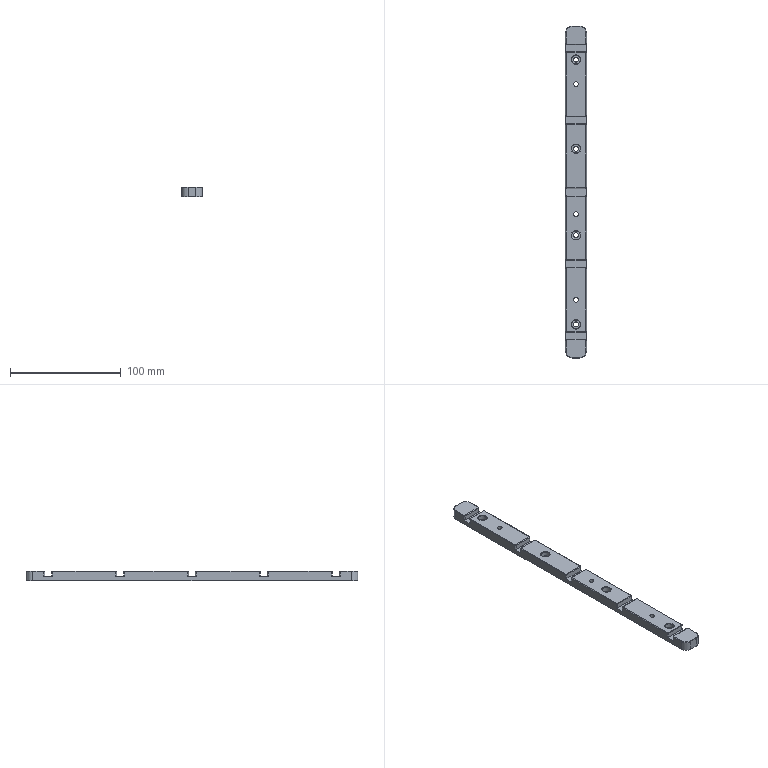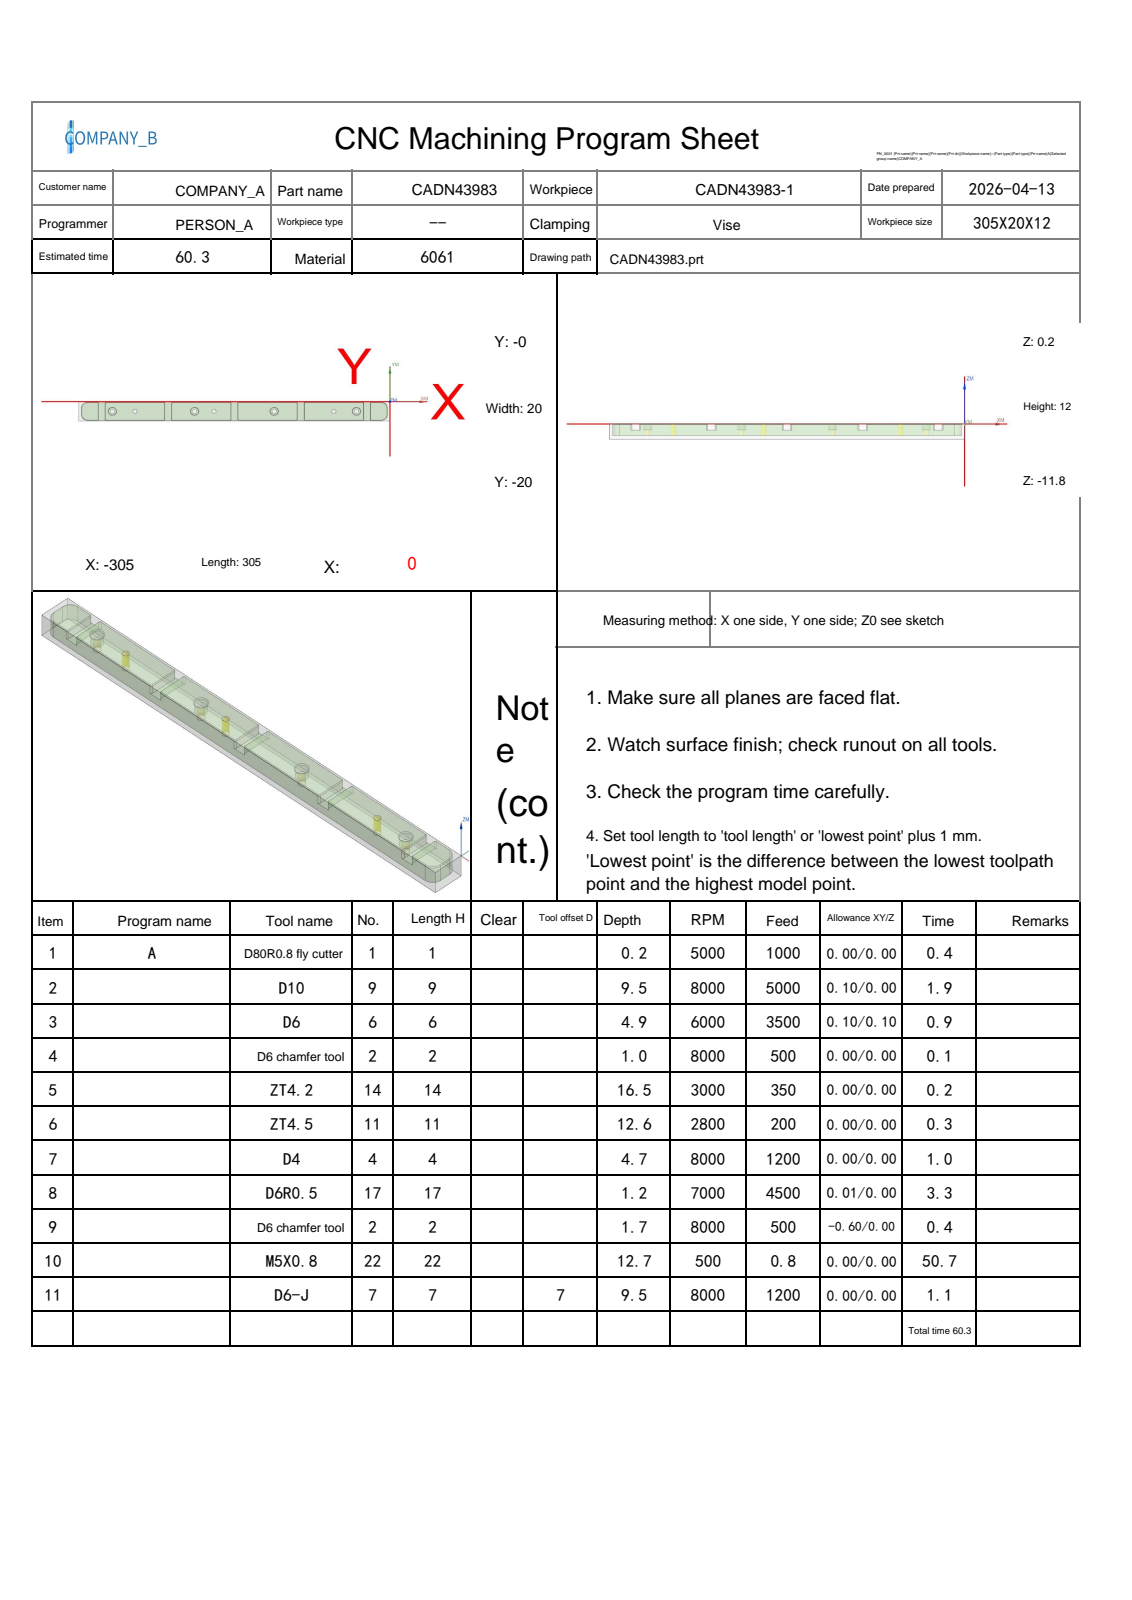NC program | NX | posted by the shop | part box 19 x 300 x 9 mm
Lines 1 to 1453 of 20188:
%
O0001
(Machine time: 109.25 MIN)
(===Total Tool:10===)
(T1=D80R0.8 fly cutter D=80.  R=0.8  D-  H01 Z=-0.   )
(T9=D10     D=10.  R=0.   D-  H09 Z=-9.3  )
(T6=D6      D=6.   R=0.   D-  H06 Z=-4.7  )
(T2=D6 chamfer tool   D=6.   R=0.   D-  H02 Z=-1.5  )
(T14=ZT4.2  D=4.2  DR_a=118 D-  H14 Z=-16.26)
(T11=ZT4.5  D=4.5  DR_a=118 D-  H11 Z=-12.35)
(T4=D4      D=4.   R=0.   D4  H04 Z=-4.5  )
(T17=D6R0.5 D=6.   R=0.5  D-  H17 Z=-1.   )
(T22=M5X0.8 D=4.2  DR_a=180 D-  H22 Z=-12.5 )
(T7=D6-J    D=6.   R=0.   D7  H07 Z=-9.3  )
G80 G90 G17 G49 G40
G91 G28 Z0
M01
N1 T01 M06
(D80R0.8 fly cutter  D=80. R=0.8 H=01 ce=0.00 di=0.00)
G00 G90 G54 X-347.5 Y-10. M03 S5000
G43 H01 Z20.
M08
Z2.
G01 Z0.0 F1000.
X-342.5
X37.5
X42.5
Z2.
G00 Z20.
G91 G28 Z0.0
M05
M09
G91 G28 Z0.0
M01
N2 T09 M06
(D10  D=10. R=0. H=09 ce=0.10 di=0.00)
G00 G90 G54 X-152.5 Y-24.6 M03 S8000
G43 H09 Z20.
M08
Z.5
G01 X-296.5 Z.335 F5000.
G02 X-307.6 Y-13.5 Z.316 I0.0 J11.1
G01 Y-6.5 Z.308
G02 X-296.5 Y4.6 Z.288 I11.1 J0.0
G01 X-8.5 Z-.041
G02 X2.6 Y-6.5 Z-.061 I0.0 J-11.1
G01 Y-13.5 Z-.069
G02 X-8.5 Y-24.6 Z-.089 I-11.1 J0.0
G01 X-296.5 Z-.418
G02 X-307.6 Y-13.5 Z-.438 I0.0 J11.1
G01 Y-6.5 Z-.446
G02 X-296.5 Y4.6 Z-.466 I11.1 J0.0
G01 X-8.5 Z-.795
G02 X2.6 Y-6.5 Z-.815 I0.0 J-11.1
G01 Y-13.5 Z-.823
G02 X-8.5 Y-24.6 Z-.843 I-11.1 J0.0
G01 X-296.5 Z-1.172
G02 X-307.6 Y-13.5 Z-1.192 I0.0 J11.1
G01 Y-6.5 Z-1.2
G02 X-296.5 Y4.6 Z-1.22 I11.1 J0.0
G01 X-8.5 Z-1.549
G02 X2.6 Y-6.5 Z-1.569 I0.0 J-11.1
G01 Y-13.5 Z-1.577
G02 X-8.5 Y-24.6 Z-1.597 I-11.1 J0.0
G01 X-296.5 Z-1.926
G02 X-307.6 Y-13.5 Z-1.946 I0.0 J11.1
G01 Y-6.5 Z-1.954
G02 X-296.5 Y4.6 Z-1.974 I11.1 J0.0
G01 X-8.5 Z-2.303
G02 X2.6 Y-6.5 Z-2.323 I0.0 J-11.1
G01 Y-13.5 Z-2.331
G02 X-8.5 Y-24.6 Z-2.351 I-11.1 J0.0
G01 X-296.5 Z-2.68
G02 X-307.6 Y-13.5 Z-2.7 I0.0 J11.1
G01 Y-6.5 Z-2.708
G02 X-296.5 Y4.6 Z-2.728 I11.1 J0.0
G01 X-8.5 Z-3.057
G02 X2.6 Y-6.5 Z-3.077 I0.0 J-11.1
G01 Y-13.5 Z-3.085
G02 X-8.5 Y-24.6 Z-3.105 I-11.1 J0.0
G01 X-296.5 Z-3.434
G02 X-307.6 Y-13.5 Z-3.454 I0.0 J11.1
G01 Y-6.5 Z-3.462
G02 X-296.5 Y4.6 Z-3.482 I11.1 J0.0
G01 X-8.5 Z-3.811
G02 X2.6 Y-6.5 Z-3.831 I0.0 J-11.1
G01 Y-13.5 Z-3.839
G02 X-8.5 Y-24.6 Z-3.859 I-11.1 J0.0
G01 X-296.5 Z-4.188
G02 X-307.6 Y-13.5 Z-4.208 I0.0 J11.1
G01 Y-6.5 Z-4.216
G02 X-296.5 Y4.6 Z-4.235 I11.1 J0.0
G01 X-8.5 Z-4.565
G02 X2.6 Y-6.5 Z-4.584 I0.0 J-11.1
G01 Y-13.5 Z-4.592
G02 X-8.5 Y-24.6 Z-4.612 I-11.1 J0.0
G01 X-296.5 Z-4.941
G02 X-307.6 Y-13.5 Z-4.961 I0.0 J11.1
G01 Y-6.5 Z-4.969
G02 X-296.5 Y4.6 Z-4.989 I11.1 J0.0
G01 X-8.5 Z-5.318
G02 X2.6 Y-6.5 Z-5.338 I0.0 J-11.1
G01 Y-13.5 Z-5.346
G02 X-8.5 Y-24.6 Z-5.366 I-11.1 J0.0
G01 X-296.5 Z-5.695
G02 X-307.6 Y-13.5 Z-5.715 I0.0 J11.1
G01 Y-6.5 Z-5.723
G02 X-296.5 Y4.6 Z-5.743 I11.1 J0.0
G01 X-8.5 Z-6.072
G02 X2.6 Y-6.5 Z-6.092 I0.0 J-11.1
G01 Y-13.5 Z-6.1
G02 X-8.5 Y-24.6 Z-6.12 I-11.1 J0.0
G01 X-296.5 Z-6.449
G02 X-307.6 Y-13.5 Z-6.469 I0.0 J11.1
G01 Y-6.5 Z-6.477
G02 X-296.5 Y4.6 Z-6.497 I11.1 J0.0
G01 X-8.5 Z-6.826
G02 X2.6 Y-6.5 Z-6.846 I0.0 J-11.1
G01 Y-13.5 Z-6.854
G02 X-8.5 Y-24.6 Z-6.874 I-11.1 J0.0
G01 X-296.5 Z-7.203
G02 X-307.6 Y-13.5 Z-7.223 I0.0 J11.1
G01 Y-6.5 Z-7.231
G02 X-296.5 Y4.6 Z-7.251 I11.1 J0.0
G01 X-8.5 Z-7.58
G02 X2.6 Y-6.5 Z-7.6 I0.0 J-11.1
G01 Y-13.5 Z-7.608
G02 X-8.5 Y-24.6 Z-7.628 I-11.1 J0.0
G01 X-296.5 Z-7.957
G02 X-307.6 Y-13.5 Z-7.977 I0.0 J11.1
G01 Y-6.5 Z-7.985
G02 X-296.5 Y4.6 Z-8.005 I11.1 J0.0
G01 X-8.5 Z-8.334
G02 X2.6 Y-6.5 Z-8.354 I0.0 J-11.1
G01 Y-13.5 Z-8.362
G02 X-8.5 Y-24.6 Z-8.382 I-11.1 J0.0
G01 X-296.5 Z-8.711
G02 X-307.6 Y-13.5 Z-8.731 I0.0 J11.1
G01 Y-6.5 Z-8.739
G02 X-296.5 Y4.6 Z-8.759 I11.1 J0.0
G01 X-8.5 Z-9.088
G02 X2.6 Y-6.5 Z-9.108 I0.0 J-11.1
G01 Y-13.5 Z-9.116
G02 X-8.5 Y-24.6 Z-9.135 I-11.1 J0.0
G01 X-152.5 Z-9.3
X-296.5
G02 X-307.6 Y-13.5 I0.0 J11.1
G01 Y-6.5
G02 X-296.5 Y4.6 I11.1 J0.0
G01 X-8.5
G02 X2.6 Y-6.5 I0.0 J-11.1
G01 Y-13.5
G02 X-8.5 Y-24.6 I-11.1 J0.0
G01 X-152.5
X-153.
Z-8.3
G00 Z20.
G91 G28 Z0.0
M05
M09
G91 G28 Z0.0
M01
N3 T06 M06
(D6  D=6. R=0. H=06 ce=0.10 di=0.10)
G00 G90 G54 X-22.5 Y5.5 M03 S6000
G43 H06 Z20.
M08
Z.108
G01 Z-.392 F3500.
Y.1
X-22.875
G02 X-22.55 Y-1.5 I-3.775 J-1.6
G01 Y-18.5
G02 X-22.875 Y-20.1 I-4.1 J0.0
G01 X-22.125
G02 X-22.45 Y-18.5 I3.775 J1.6
G01 Y-1.5
G02 X-22.125 Y.1 I4.1 J0.0
G01 X-22.5
X-22.875
X-22.828 Y-.016
Z.108
G00 Z.5
X-22.5 Y5.5
Z-.283
G01 Z-.783
Y.1
X-22.875
G02 X-22.55 Y-1.5 I-3.775 J-1.6
G01 Y-18.5
G02 X-22.875 Y-20.1 I-4.1 J0.0
G01 X-22.125
G02 X-22.45 Y-18.5 I3.775 J1.6
G01 Y-1.5
G02 X-22.125 Y.1 I4.1 J0.0
G01 X-22.5
X-22.875
X-22.828 Y-.016
Z-.283
G00 Z.108
X-22.5 Y5.5
Z-.675
G01 Z-1.175
Y.1
X-22.875
G02 X-22.55 Y-1.5 I-3.775 J-1.6
G01 Y-18.5
G02 X-22.875 Y-20.1 I-4.1 J0.0
G01 X-22.125
G02 X-22.45 Y-18.5 I3.775 J1.6
G01 Y-1.5
G02 X-22.125 Y.1 I4.1 J0.0
G01 X-22.5
X-22.875
X-22.828 Y-.016
Z-.675
G00 Z-.283
X-22.5 Y5.5
Z-1.067
G01 Z-1.567
Y.1
X-22.875
G02 X-22.55 Y-1.5 I-3.775 J-1.6
G01 Y-18.5
G02 X-22.875 Y-20.1 I-4.1 J0.0
G01 X-22.125
G02 X-22.45 Y-18.5 I3.775 J1.6
G01 Y-1.5
G02 X-22.125 Y.1 I4.1 J0.0
G01 X-22.5
X-22.875
X-22.828 Y-.016
Z-1.067
G00 Z-.675
X-22.5 Y5.5
Z-1.458
G01 Z-1.958
Y.1
X-22.875
G02 X-22.55 Y-1.5 I-3.775 J-1.6
G01 Y-18.5
G02 X-22.875 Y-20.1 I-4.1 J0.0
G01 X-22.125
G02 X-22.45 Y-18.5 I3.775 J1.6
G01 Y-1.5
G02 X-22.125 Y.1 I4.1 J0.0
G01 X-22.5
X-22.875
X-22.828 Y-.016
Z-1.458
G00 Z-1.067
X-22.5 Y5.5
Z-1.85
G01 Z-2.35
Y.1
X-22.875
G02 X-22.55 Y-1.5 I-3.775 J-1.6
G01 Y-18.5
G02 X-22.875 Y-20.1 I-4.1 J0.0
G01 X-22.125
G02 X-22.45 Y-18.5 I3.775 J1.6
G01 Y-1.5
G02 X-22.125 Y.1 I4.1 J0.0
G01 X-22.5
X-22.875
X-22.828 Y-.016
Z-1.85
G00 Z-1.458
X-22.5 Y5.5
Z-2.242
G01 Z-2.742
Y.1
X-22.875
G02 X-22.55 Y-1.5 I-3.775 J-1.6
G01 Y-18.5
G02 X-22.875 Y-20.1 I-4.1 J0.0
G01 X-22.125
G02 X-22.45 Y-18.5 I3.775 J1.6
G01 Y-1.5
G02 X-22.125 Y.1 I4.1 J0.0
G01 X-22.5
X-22.875
X-22.828 Y-.016
Z-2.242
G00 Z-1.85
X-22.5 Y5.5
Z-2.633
G01 Z-3.133
Y.1
X-22.875
G02 X-22.55 Y-1.5 I-3.775 J-1.6
G01 Y-18.5
G02 X-22.875 Y-20.1 I-4.1 J0.0
G01 X-22.125
G02 X-22.45 Y-18.5 I3.775 J1.6
G01 Y-1.5
G02 X-22.125 Y.1 I4.1 J0.0
G01 X-22.5
X-22.875
X-22.828 Y-.016
Z-2.633
G00 Z-2.242
X-22.5 Y5.5
Z-3.025
G01 Z-3.525
Y.1
X-22.875
G02 X-22.55 Y-1.5 I-3.775 J-1.6
G01 Y-18.5
G02 X-22.875 Y-20.1 I-4.1 J0.0
G01 X-22.125
G02 X-22.45 Y-18.5 I3.775 J1.6
G01 Y-1.5
G02 X-22.125 Y.1 I4.1 J0.0
G01 X-22.5
X-22.875
X-22.828 Y-.016
Z-3.025
G00 Z-2.633
X-22.5 Y5.5
Z-3.417
G01 Z-3.917
Y.1
X-22.875
G02 X-22.55 Y-1.5 I-3.775 J-1.6
G01 Y-18.5
G02 X-22.875 Y-20.1 I-4.1 J0.0
G01 X-22.125
G02 X-22.45 Y-18.5 I3.775 J1.6
G01 Y-1.5
G02 X-22.125 Y.1 I4.1 J0.0
G01 X-22.5
X-22.875
X-22.828 Y-.016
Z-3.417
G00 Z-3.025
X-22.5 Y5.5
Z-3.808
G01 Z-4.308
Y.1
X-22.875
G02 X-22.55 Y-1.5 I-3.775 J-1.6
G01 Y-18.5
G02 X-22.875 Y-20.1 I-4.1 J0.0
G01 X-22.125
G02 X-22.45 Y-18.5 I3.775 J1.6
G01 Y-1.5
G02 X-22.125 Y.1 I4.1 J0.0
G01 X-22.5
X-22.875
X-22.828 Y-.016
Z-3.808
G00 Z-3.417
X-22.5 Y5.5
Z-4.2
G01 Z-4.7
Y.1
X-22.875
G02 X-22.55 Y-1.5 I-3.775 J-1.6
G01 Y-18.5
G02 X-22.875 Y-20.1 I-4.1 J0.0
G01 X-22.125
G02 X-22.45 Y-18.5 I3.775 J1.6
G01 Y-1.5
G02 X-22.125 Y.1 I4.1 J0.0
G01 X-22.5
X-22.875
X-22.828 Y-.016
Z-4.2
G00 Z20.
X-87.5 Y5.5
Z.108
G01 Z-.392
Y.1
X-87.875
G02 X-87.55 Y-1.5 I-3.775 J-1.6
G01 Y-18.5
G02 X-87.875 Y-20.1 I-4.1 J0.0
G01 X-87.125
G02 X-87.45 Y-18.5 I3.775 J1.6
G01 Y-1.5
G02 X-87.125 Y.1 I4.1 J0.0
G01 X-87.5
X-87.875
X-87.828 Y-.016
Z.108
G00 Z.5
X-87.5 Y5.5
Z-.283
G01 Z-.783
Y.1
X-87.875
G02 X-87.55 Y-1.5 I-3.775 J-1.6
G01 Y-18.5
G02 X-87.875 Y-20.1 I-4.1 J0.0
G01 X-87.125
G02 X-87.45 Y-18.5 I3.775 J1.6
G01 Y-1.5
G02 X-87.125 Y.1 I4.1 J0.0
G01 X-87.5
X-87.875
X-87.828 Y-.016
Z-.283
G00 Z.108
X-87.5 Y5.5
Z-.675
G01 Z-1.175
Y.1
X-87.875
G02 X-87.55 Y-1.5 I-3.775 J-1.6
G01 Y-18.5
G02 X-87.875 Y-20.1 I-4.1 J0.0
G01 X-87.125
G02 X-87.45 Y-18.5 I3.775 J1.6
G01 Y-1.5
G02 X-87.125 Y.1 I4.1 J0.0
G01 X-87.5
X-87.875
X-87.828 Y-.016
Z-.675
G00 Z-.283
X-87.5 Y5.5
Z-1.067
G01 Z-1.567
Y.1
X-87.875
G02 X-87.55 Y-1.5 I-3.775 J-1.6
G01 Y-18.5
G02 X-87.875 Y-20.1 I-4.1 J0.0
G01 X-87.125
G02 X-87.45 Y-18.5 I3.775 J1.6
G01 Y-1.5
G02 X-87.125 Y.1 I4.1 J0.0
G01 X-87.5
X-87.875
X-87.828 Y-.016
Z-1.067
G00 Z-.675
X-87.5 Y5.5
Z-1.458
G01 Z-1.958
Y.1
X-87.875
G02 X-87.55 Y-1.5 I-3.775 J-1.6
G01 Y-18.5
G02 X-87.875 Y-20.1 I-4.1 J0.0
G01 X-87.125
G02 X-87.45 Y-18.5 I3.775 J1.6
G01 Y-1.5
G02 X-87.125 Y.1 I4.1 J0.0
G01 X-87.5
X-87.875
X-87.828 Y-.016
Z-1.458
G00 Z-1.067
X-87.5 Y5.5
Z-1.85
G01 Z-2.35
Y.1
X-87.875
G02 X-87.55 Y-1.5 I-3.775 J-1.6
G01 Y-18.5
G02 X-87.875 Y-20.1 I-4.1 J0.0
G01 X-87.125
G02 X-87.45 Y-18.5 I3.775 J1.6
G01 Y-1.5
G02 X-87.125 Y.1 I4.1 J0.0
G01 X-87.5
X-87.875
X-87.828 Y-.016
Z-1.85
G00 Z-1.458
X-87.5 Y5.5
Z-2.242
G01 Z-2.742
Y.1
X-87.875
G02 X-87.55 Y-1.5 I-3.775 J-1.6
G01 Y-18.5
G02 X-87.875 Y-20.1 I-4.1 J0.0
G01 X-87.125
G02 X-87.45 Y-18.5 I3.775 J1.6
G01 Y-1.5
G02 X-87.125 Y.1 I4.1 J0.0
G01 X-87.5
X-87.875
X-87.828 Y-.016
Z-2.242
G00 Z-1.85
X-87.5 Y5.5
Z-2.633
G01 Z-3.133
Y.1
X-87.875
G02 X-87.55 Y-1.5 I-3.775 J-1.6
G01 Y-18.5
G02 X-87.875 Y-20.1 I-4.1 J0.0
G01 X-87.125
G02 X-87.45 Y-18.5 I3.775 J1.6
G01 Y-1.5
G02 X-87.125 Y.1 I4.1 J0.0
G01 X-87.5
X-87.875
X-87.828 Y-.016
Z-2.633
G00 Z-2.242
X-87.5 Y5.5
Z-3.025
G01 Z-3.525
Y.1
X-87.875
G02 X-87.55 Y-1.5 I-3.775 J-1.6
G01 Y-18.5
G02 X-87.875 Y-20.1 I-4.1 J0.0
G01 X-87.125
G02 X-87.45 Y-18.5 I3.775 J1.6
G01 Y-1.5
G02 X-87.125 Y.1 I4.1 J0.0
G01 X-87.5
X-87.875
X-87.828 Y-.016
Z-3.025
G00 Z-2.633
X-87.5 Y5.5
Z-3.417
G01 Z-3.917
Y.1
X-87.875
G02 X-87.55 Y-1.5 I-3.775 J-1.6
G01 Y-18.5
G02 X-87.875 Y-20.1 I-4.1 J0.0
G01 X-87.125
G02 X-87.45 Y-18.5 I3.775 J1.6
G01 Y-1.5
G02 X-87.125 Y.1 I4.1 J0.0
G01 X-87.5
X-87.875
X-87.828 Y-.016
Z-3.417
G00 Z-3.025
X-87.5 Y5.5
Z-3.808
G01 Z-4.308
Y.1
X-87.875
G02 X-87.55 Y-1.5 I-3.775 J-1.6
G01 Y-18.5
G02 X-87.875 Y-20.1 I-4.1 J0.0
G01 X-87.125
G02 X-87.45 Y-18.5 I3.775 J1.6
G01 Y-1.5
G02 X-87.125 Y.1 I4.1 J0.0
G01 X-87.5
X-87.875
X-87.828 Y-.016
Z-3.808
G00 Z-3.417
X-87.5 Y5.5
Z-4.2
G01 Z-4.7
Y.1
X-87.875
G02 X-87.55 Y-1.5 I-3.775 J-1.6
G01 Y-18.5
G02 X-87.875 Y-20.1 I-4.1 J0.0
G01 X-87.125
G02 X-87.45 Y-18.5 I3.775 J1.6
G01 Y-1.5
G02 X-87.125 Y.1 I4.1 J0.0
G01 X-87.5
X-87.875
X-87.828 Y-.016
Z-4.2
G00 Z20.
X-152.5 Y5.5
Z.108
G01 Z-.392
Y.1
X-152.875
G02 X-152.55 Y-1.5 I-3.775 J-1.6
G01 Y-18.5
G02 X-152.875 Y-20.1 I-4.1 J0.0
G01 X-152.125
G02 X-152.45 Y-18.5 I3.775 J1.6
G01 Y-1.5
G02 X-152.125 Y.1 I4.1 J0.0
G01 X-152.5
X-152.875
X-152.828 Y-.016
Z.108
G00 Z.5
X-152.5 Y5.5
Z-.283
G01 Z-.783
Y.1
X-152.875
G02 X-152.55 Y-1.5 I-3.775 J-1.6
G01 Y-18.5
G02 X-152.875 Y-20.1 I-4.1 J0.0
G01 X-152.125
G02 X-152.45 Y-18.5 I3.775 J1.6
G01 Y-1.5
G02 X-152.125 Y.1 I4.1 J0.0
G01 X-152.5
X-152.875
X-152.828 Y-.016
Z-.283
G00 Z.108
X-152.5 Y5.5
Z-.675
G01 Z-1.175
Y.1
X-152.875
G02 X-152.55 Y-1.5 I-3.775 J-1.6
G01 Y-18.5
G02 X-152.875 Y-20.1 I-4.1 J0.0
G01 X-152.125
G02 X-152.45 Y-18.5 I3.775 J1.6
G01 Y-1.5
G02 X-152.125 Y.1 I4.1 J0.0
G01 X-152.5
X-152.875
X-152.828 Y-.016
Z-.675
G00 Z-.283
X-152.5 Y5.5
Z-1.067
G01 Z-1.567
Y.1
X-152.875
G02 X-152.55 Y-1.5 I-3.775 J-1.6
G01 Y-18.5
G02 X-152.875 Y-20.1 I-4.1 J0.0
G01 X-152.125
G02 X-152.45 Y-18.5 I3.775 J1.6
G01 Y-1.5
G02 X-152.125 Y.1 I4.1 J0.0
G01 X-152.5
X-152.875
X-152.828 Y-.016
Z-1.067
G00 Z-.675
X-152.5 Y5.5
Z-1.458
G01 Z-1.958
Y.1
X-152.875
G02 X-152.55 Y-1.5 I-3.775 J-1.6
G01 Y-18.5
G02 X-152.875 Y-20.1 I-4.1 J0.0
G01 X-152.125
G02 X-152.45 Y-18.5 I3.775 J1.6
G01 Y-1.5
G02 X-152.125 Y.1 I4.1 J0.0
G01 X-152.5
X-152.875
X-152.828 Y-.016
Z-1.458
G00 Z-1.067
X-152.5 Y5.5
Z-1.85
G01 Z-2.35
Y.1
X-152.875
G02 X-152.55 Y-1.5 I-3.775 J-1.6
G01 Y-18.5
G02 X-152.875 Y-20.1 I-4.1 J0.0
G01 X-152.125
G02 X-152.45 Y-18.5 I3.775 J1.6
G01 Y-1.5
G02 X-152.125 Y.1 I4.1 J0.0
G01 X-152.5
X-152.875
X-152.828 Y-.016
Z-1.85
G00 Z-1.458
X-152.5 Y5.5
Z-2.242
G01 Z-2.742
Y.1
X-152.875
G02 X-152.55 Y-1.5 I-3.775 J-1.6
G01 Y-18.5
G02 X-152.875 Y-20.1 I-4.1 J0.0
G01 X-152.125
G02 X-152.45 Y-18.5 I3.775 J1.6
G01 Y-1.5
G02 X-152.125 Y.1 I4.1 J0.0
G01 X-152.5
X-152.875
X-152.828 Y-.016
Z-2.242
G00 Z-1.85
X-152.5 Y5.5
Z-2.633
G01 Z-3.133
Y.1
X-152.875
G02 X-152.55 Y-1.5 I-3.775 J-1.6
G01 Y-18.5
G02 X-152.875 Y-20.1 I-4.1 J0.0
G01 X-152.125
G02 X-152.45 Y-18.5 I3.775 J1.6
G01 Y-1.5
G02 X-152.125 Y.1 I4.1 J0.0
G01 X-152.5
X-152.875
X-152.828 Y-.016
Z-2.633
G00 Z-2.242
X-152.5 Y5.5
Z-3.025
G01 Z-3.525
Y.1
X-152.875
G02 X-152.55 Y-1.5 I-3.775 J-1.6
G01 Y-18.5
G02 X-152.875 Y-20.1 I-4.1 J0.0
G01 X-152.125
G02 X-152.45 Y-18.5 I3.775 J1.6
G01 Y-1.5
G02 X-152.125 Y.1 I4.1 J0.0
G01 X-152.5
X-152.875
X-152.828 Y-.016
Z-3.025
G00 Z-2.633
X-152.5 Y5.5
Z-3.417
G01 Z-3.917
Y.1
X-152.875
G02 X-152.55 Y-1.5 I-3.775 J-1.6
G01 Y-18.5
G02 X-152.875 Y-20.1 I-4.1 J0.0
G01 X-152.125
G02 X-152.45 Y-18.5 I3.775 J1.6
G01 Y-1.5
G02 X-152.125 Y.1 I4.1 J0.0
G01 X-152.5
X-152.875
X-152.828 Y-.016
Z-3.417
G00 Z-3.025
X-152.5 Y5.5
Z-3.808
G01 Z-4.308
Y.1
X-152.875
G02 X-152.55 Y-1.5 I-3.775 J-1.6
G01 Y-18.5
G02 X-152.875 Y-20.1 I-4.1 J0.0
G01 X-152.125
G02 X-152.45 Y-18.5 I3.775 J1.6
G01 Y-1.5
G02 X-152.125 Y.1 I4.1 J0.0
G01 X-152.5
X-152.875
X-152.828 Y-.016
Z-3.808
G00 Z-3.417
X-152.5 Y5.5
Z-4.2
G01 Z-4.7
Y.1
X-152.875
G02 X-152.55 Y-1.5 I-3.775 J-1.6
G01 Y-18.5
G02 X-152.875 Y-20.1 I-4.1 J0.0
G01 X-152.125
G02 X-152.45 Y-18.5 I3.775 J1.6
G01 Y-1.5
G02 X-152.125 Y.1 I4.1 J0.0
G01 X-152.5
X-152.875
X-152.828 Y-.016
Z-4.2
G00 Z20.
X-217.5 Y5.5
Z.108
G01 Z-.392
Y.1
X-217.875
G02 X-217.55 Y-1.5 I-3.775 J-1.6
G01 Y-18.5
G02 X-217.875 Y-20.1 I-4.1 J0.0
G01 X-217.125
G02 X-217.45 Y-18.5 I3.775 J1.6
G01 Y-1.5
G02 X-217.125 Y.1 I4.1 J0.0
G01 X-217.5
X-217.875
X-217.828 Y-.016
Z.108
G00 Z.5
X-217.5 Y5.5
Z-.283
G01 Z-.783
Y.1
X-217.875
G02 X-217.55 Y-1.5 I-3.775 J-1.6
G01 Y-18.5
G02 X-217.875 Y-20.1 I-4.1 J0.0
G01 X-217.125
G02 X-217.45 Y-18.5 I3.775 J1.6
G01 Y-1.5
G02 X-217.125 Y.1 I4.1 J0.0
G01 X-217.5
X-217.875
X-217.828 Y-.016
Z-.283
G00 Z.108
X-217.5 Y5.5
Z-.675
G01 Z-1.175
Y.1
X-217.875
G02 X-217.55 Y-1.5 I-3.775 J-1.6
G01 Y-18.5
G02 X-217.875 Y-20.1 I-4.1 J0.0
G01 X-217.125
G02 X-217.45 Y-18.5 I3.775 J1.6
G01 Y-1.5
G02 X-217.125 Y.1 I4.1 J0.0
G01 X-217.5
X-217.875
X-217.828 Y-.016
Z-.675
G00 Z-.283
X-217.5 Y5.5
Z-1.067
G01 Z-1.567
Y.1
X-217.875
G02 X-217.55 Y-1.5 I-3.775 J-1.6
G01 Y-18.5
G02 X-217.875 Y-20.1 I-4.1 J0.0
G01 X-217.125
G02 X-217.45 Y-18.5 I3.775 J1.6
G01 Y-1.5
G02 X-217.125 Y.1 I4.1 J0.0
G01 X-217.5
X-217.875
X-217.828 Y-.016
Z-1.067
G00 Z-.675
X-217.5 Y5.5
Z-1.458
G01 Z-1.958
Y.1
X-217.875
G02 X-217.55 Y-1.5 I-3.775 J-1.6
G01 Y-18.5
G02 X-217.875 Y-20.1 I-4.1 J0.0
G01 X-217.125
G02 X-217.45 Y-18.5 I3.775 J1.6
G01 Y-1.5
G02 X-217.125 Y.1 I4.1 J0.0
G01 X-217.5
X-217.875
X-217.828 Y-.016
Z-1.458
G00 Z-1.067
X-217.5 Y5.5
Z-1.85
G01 Z-2.35
Y.1
X-217.875
G02 X-217.55 Y-1.5 I-3.775 J-1.6
G01 Y-18.5
G02 X-217.875 Y-20.1 I-4.1 J0.0
G01 X-217.125
G02 X-217.45 Y-18.5 I3.775 J1.6
G01 Y-1.5
G02 X-217.125 Y.1 I4.1 J0.0
G01 X-217.5
X-217.875
X-217.828 Y-.016
Z-1.85
G00 Z-1.458
X-217.5 Y5.5
Z-2.242
G01 Z-2.742
Y.1
X-217.875
G02 X-217.55 Y-1.5 I-3.775 J-1.6
G01 Y-18.5
G02 X-217.875 Y-20.1 I-4.1 J0.0
G01 X-217.125
G02 X-217.45 Y-18.5 I3.775 J1.6
G01 Y-1.5
G02 X-217.125 Y.1 I4.1 J0.0
G01 X-217.5
X-217.875
X-217.828 Y-.016
Z-2.242
G00 Z-1.85
X-217.5 Y5.5
Z-2.633
G01 Z-3.133
Y.1
X-217.875
G02 X-217.55 Y-1.5 I-3.775 J-1.6
G01 Y-18.5
G02 X-217.875 Y-20.1 I-4.1 J0.0
G01 X-217.125
G02 X-217.45 Y-18.5 I3.775 J1.6
G01 Y-1.5
G02 X-217.125 Y.1 I4.1 J0.0
G01 X-217.5
X-217.875
X-217.828 Y-.016
Z-2.633
G00 Z-2.242
X-217.5 Y5.5
Z-3.025
G01 Z-3.525
Y.1
X-217.875
G02 X-217.55 Y-1.5 I-3.775 J-1.6
G01 Y-18.5
G02 X-217.875 Y-20.1 I-4.1 J0.0
G01 X-217.125
G02 X-217.45 Y-18.5 I3.775 J1.6
G01 Y-1.5
G02 X-217.125 Y.1 I4.1 J0.0
G01 X-217.5
X-217.875
X-217.828 Y-.016
Z-3.025
G00 Z-2.633
X-217.5 Y5.5
Z-3.417
G01 Z-3.917
Y.1
X-217.875
G02 X-217.55 Y-1.5 I-3.775 J-1.6
G01 Y-18.5
G02 X-217.875 Y-20.1 I-4.1 J0.0
G01 X-217.125
G02 X-217.45 Y-18.5 I3.775 J1.6
G01 Y-1.5
G02 X-217.125 Y.1 I4.1 J0.0
G01 X-217.5
X-217.875
X-217.828 Y-.016
Z-3.417
G00 Z-3.025
X-217.5 Y5.5
Z-3.808
G01 Z-4.308
Y.1
X-217.875
G02 X-217.55 Y-1.5 I-3.775 J-1.6
G01 Y-18.5
G02 X-217.875 Y-20.1 I-4.1 J0.0
G01 X-217.125
G02 X-217.45 Y-18.5 I3.775 J1.6
G01 Y-1.5
G02 X-217.125 Y.1 I4.1 J0.0
G01 X-217.5
X-217.875
X-217.828 Y-.016
Z-3.808
G00 Z-3.417
X-217.5 Y5.5
Z-4.2
G01 Z-4.7
Y.1
X-217.875
G02 X-217.55 Y-1.5 I-3.775 J-1.6
G01 Y-18.5
G02 X-217.875 Y-20.1 I-4.1 J0.0
G01 X-217.125
G02 X-217.45 Y-18.5 I3.775 J1.6
G01 Y-1.5
G02 X-217.125 Y.1 I4.1 J0.0
G01 X-217.5
X-217.875
X-217.828 Y-.016
Z-4.2
G00 Z20.
X-282.5 Y5.5
Z.108
G01 Z-.392
Y.1
X-282.875
G02 X-282.55 Y-1.5 I-3.775 J-1.6
G01 Y-18.5
G02 X-282.875 Y-20.1 I-4.1 J0.0
G01 X-282.125
G02 X-282.45 Y-18.5 I3.775 J1.6
G01 Y-1.5
G02 X-282.125 Y.1 I4.1 J0.0
G01 X-282.5
X-282.875
X-282.828 Y-.016
Z.108
G00 Z.5
X-282.5 Y5.5
Z-.283
G01 Z-.783
Y.1
X-282.875
G02 X-282.55 Y-1.5 I-3.775 J-1.6
G01 Y-18.5
G02 X-282.875 Y-20.1 I-4.1 J0.0
G01 X-282.125
G02 X-282.45 Y-18.5 I3.775 J1.6
G01 Y-1.5
G02 X-282.125 Y.1 I4.1 J0.0
G01 X-282.5
X-282.875
X-282.828 Y-.016
Z-.283
G00 Z.108
X-282.5 Y5.5
Z-.675
G01 Z-1.175
Y.1
X-282.875
G02 X-282.55 Y-1.5 I-3.775 J-1.6
G01 Y-18.5
G02 X-282.875 Y-20.1 I-4.1 J0.0
G01 X-282.125
G02 X-282.45 Y-18.5 I3.775 J1.6
G01 Y-1.5
G02 X-282.125 Y.1 I4.1 J0.0
G01 X-282.5
X-282.875
X-282.828 Y-.016
Z-.675
G00 Z-.283
X-282.5 Y5.5
Z-1.067
G01 Z-1.567
Y.1
X-282.875
G02 X-282.55 Y-1.5 I-3.775 J-1.6
G01 Y-18.5
G02 X-282.875 Y-20.1 I-4.1 J0.0
G01 X-282.125
G02 X-282.45 Y-18.5 I3.775 J1.6
G01 Y-1.5
G02 X-282.125 Y.1 I4.1 J0.0
G01 X-282.5
X-282.875
X-282.828 Y-.016
Z-1.067
G00 Z-.675
X-282.5 Y5.5
Z-1.458
G01 Z-1.958
Y.1
X-282.875
G02 X-282.55 Y-1.5 I-3.775 J-1.6
G01 Y-18.5
G02 X-282.875 Y-20.1 I-4.1 J0.0
G01 X-282.125
G02 X-282.45 Y-18.5 I3.775 J1.6
G01 Y-1.5
G02 X-282.125 Y.1 I4.1 J0.0
G01 X-282.5
X-282.875
X-282.828 Y-.016
Z-1.458
G00 Z-1.067
X-282.5 Y5.5
Z-1.85
G01 Z-2.35
Y.1
X-282.875
G02 X-282.55 Y-1.5 I-3.775 J-1.6
G01 Y-18.5
G02 X-282.875 Y-20.1 I-4.1 J0.0
G01 X-282.125
G02 X-282.45 Y-18.5 I3.775 J1.6
G01 Y-1.5
G02 X-282.125 Y.1 I4.1 J0.0
G01 X-282.5
X-282.875
X-282.828 Y-.016
Z-1.85
G00 Z-1.458
X-282.5 Y5.5
Z-2.242
G01 Z-2.742
Y.1
X-282.875
G02 X-282.55 Y-1.5 I-3.775 J-1.6
G01 Y-18.5
G02 X-282.875 Y-20.1 I-4.1 J0.0
G01 X-282.125
G02 X-282.45 Y-18.5 I3.775 J1.6
G01 Y-1.5
G02 X-282.125 Y.1 I4.1 J0.0
G01 X-282.5
X-282.875
X-282.828 Y-.016
Z-2.242
G00 Z-1.85
X-282.5 Y5.5
Z-2.633
G01 Z-3.133
Y.1
X-282.875
G02 X-282.55 Y-1.5 I-3.775 J-1.6
G01 Y-18.5
G02 X-282.875 Y-20.1 I-4.1 J0.0
G01 X-282.125
G02 X-282.45 Y-18.5 I3.775 J1.6
G01 Y-1.5
G02 X-282.125 Y.1 I4.1 J0.0
G01 X-282.5
X-282.875
X-282.828 Y-.016
Z-2.633
G00 Z-2.242
X-282.5 Y5.5
Z-3.025
G01 Z-3.525
Y.1
X-282.875
G02 X-282.55 Y-1.5 I-3.775 J-1.6
G01 Y-18.5
G02 X-282.875 Y-20.1 I-4.1 J0.0
G01 X-282.125
G02 X-282.45 Y-18.5 I3.775 J1.6
G01 Y-1.5
G02 X-282.125 Y.1 I4.1 J0.0
G01 X-282.5
X-282.875
X-282.828 Y-.016
Z-3.025
G00 Z-2.633
X-282.5 Y5.5
Z-3.417
G01 Z-3.917
Y.1
X-282.875
G02 X-282.55 Y-1.5 I-3.775 J-1.6
G01 Y-18.5
G02 X-282.875 Y-20.1 I-4.1 J0.0
G01 X-282.125
G02 X-282.45 Y-18.5 I3.775 J1.6
G01 Y-1.5
G02 X-282.125 Y.1 I4.1 J0.0
G01 X-282.5
X-282.875
X-282.828 Y-.016
Z-3.417
G00 Z-3.025
X-282.5 Y5.5
Z-3.808
G01 Z-4.308
Y.1
X-282.875
G02 X-282.55 Y-1.5 I-3.775 J-1.6
G01 Y-18.5
G02 X-282.875 Y-20.1 I-4.1 J0.0
G01 X-282.125
G02 X-282.45 Y-18.5 I3.775 J1.6
G01 Y-1.5
G02 X-282.125 Y.1 I4.1 J0.0
G01 X-282.5
X-282.875
X-282.828 Y-.016
Z-3.808
G00 Z-3.417
X-282.5 Y5.5
Z-4.2
G01 Z-4.7
Y.1
X-282.875
G02 X-282.55 Y-1.5 I-3.775 J-1.6
G01 Y-18.5
G02 X-282.875 Y-20.1 I-4.1 J0.0
G01 X-282.125
G02 X-282.45 Y-18.5 I3.775 J1.6
G01 Y-1.5
G02 X-282.125 Y.1 I4.1 J0.0
G01 X-282.5
X-282.875
X-282.828 Y-.016
Z-4.2
G00 Z20.
G91 G28 Z0.0
M05
M09
G91 G28 Z0.0
M01
N4 T02 M06
(D6 chamfer tool  D=6. R=0. H=02 ce=0.00 di=0.10)
G00 G90 G54 X-32.9 Y-10. M03 S8000
G43 H02 Z20.
M08
G98 G81 X-32.9 Y-10. Z-.8 R1. F500.
X-55.
X-113.5
X-172.5
X-191.5
X-250.
X-272.1
G80
G00 Z20.
G91 G28 Z0.0
M05
M09
G91 G28 Z0.0
M01
N5 T14 M06
(ZT4.2 D=4.2 DR_a=118 H=14)
G00 G90 G54 X-55. Y-10. M03 S3000
G43 H14 Z20.
M08
G98 G83 X-55. Y-10. Z-16.262 R1. F350. Q3.
X-172.5
X-250.
G80
G00 Z20.
G91 G28 Z0.0
M05
M09
G91 G28 Z0.0
M01
N6 T11 M06
(ZT4.5 D=4.5 DR_a=118 H=11)
G00 G90 G54 X-32.9 Y-10. M03 S2800
G43 H11 Z20.
M08
G98 G83 X-32.9 Y-10. Z-12.352 R1. F200. Q2.
X-113.5
X-191.5
X-272.1
G80
G00 Z20.
G91 G28 Z0.0
M05
M09
G91 G28 Z0.0
M01
N7 T04 M06
(D4  D=4. R=0. H=04 ce=0.10 di=0.00)
G00 G90 G54 X-113.5 Y-10. M03 S8000
G43 H04 Z20.
M08
Z1.
G03 X-114.325 Y-10.825 I0.0 J-.825 F1200.
X-113.5 Y-11.65 I.825 J0.0
X-113.5 Y-11.65 Z.7 I0.0 J1.65
X-113.5 Y-11.65 Z.4 I0.0 J1.65
X-113.5 Y-11.65 Z.1 I0.0 J1.65
X-113.5 Y-11.65 Z-.2 I0.0 J1.65
X-113.5 Y-11.65 Z-.5 I0.0 J1.65
X-113.5 Y-11.65 Z-.8 I0.0 J1.65
X-113.5 Y-11.65 Z-1.1 I0.0 J1.65
X-113.5 Y-11.65 Z-1.4 I0.0 J1.65
X-113.5 Y-11.65 Z-1.7 I0.0 J1.65
X-113.5 Y-11.65 Z-2. I0.0 J1.65
X-113.5 Y-11.65 Z-2.3 I0.0 J1.65
X-113.5 Y-11.65 Z-2.6 I0.0 J1.65
X-113.5 Y-11.65 Z-2.9 I0.0 J1.65
X-113.5 Y-11.65 Z-3.2 I0.0 J1.65
X-113.5 Y-11.65 Z-3.5 I0.0 J1.65
X-113.5 Y-11.65 Z-3.8 I0.0 J1.65
X-113.5 Y-11.65 Z-4.1 I0.0 J1.65
X-113.5 Y-11.65 Z-4.4 I0.0 J1.65
X-112.071 Y-9.175 Z-4.5 I0.0 J1.65
X-113.5 Y-8.35 I-1.429 J-.825
X-115.15 Y-10. I0.0 J-1.65
X-113.5 Y-11.65 I1.65 J0.0
X-111.85 Y-10. I0.0 J1.65
X-112.071 Y-9.175 I-1.65 J0.0
X-112.786 Y-8.763 I-.714 J-.413
X-113.611 Y-9.588 I0.0 J-.825
X-113.5 Y-10. I.825 J0.0
G00 Z20.
X-32.9
Z1.
G03 X-33.725 Y-10.825 I0.0 J-.825
X-32.9 Y-11.65 I.825 J0.0
X-32.9 Y-11.65 Z.7 I0.0 J1.65
X-32.9 Y-11.65 Z.4 I0.0 J1.65
X-32.9 Y-11.65 Z.1 I0.0 J1.65
X-32.9 Y-11.65 Z-.2 I0.0 J1.65
X-32.9 Y-11.65 Z-.5 I0.0 J1.65
X-32.9 Y-11.65 Z-.8 I0.0 J1.65
X-32.9 Y-11.65 Z-1.1 I0.0 J1.65
X-32.9 Y-11.65 Z-1.4 I0.0 J1.65
X-32.9 Y-11.65 Z-1.7 I0.0 J1.65
X-32.9 Y-11.65 Z-2. I0.0 J1.65
X-32.9 Y-11.65 Z-2.3 I0.0 J1.65
X-32.9 Y-11.65 Z-2.6 I0.0 J1.65
X-32.9 Y-11.65 Z-2.9 I0.0 J1.65
X-32.9 Y-11.65 Z-3.2 I0.0 J1.65
X-32.9 Y-11.65 Z-3.5 I0.0 J1.65
X-32.9 Y-11.65 Z-3.8 I0.0 J1.65
X-32.9 Y-11.65 Z-4.1 I0.0 J1.65
X-32.9 Y-11.65 Z-4.4 I0.0 J1.65
X-31.471 Y-9.175 Z-4.5 I0.0 J1.65
X-32.9 Y-8.35 I-1.429 J-.825
X-34.55 Y-10. I0.0 J-1.65
X-32.9 Y-11.65 I1.65 J0.0
X-31.25 Y-10. I0.0 J1.65
X-31.471 Y-9.175 I-1.65 J0.0
X-32.186 Y-8.763 I-.714 J-.413
X-33.011 Y-9.588 I0.0 J-.825
X-32.9 Y-10. I.825 J0.0
G00 Z20.
X-191.5
Z1.
G03 X-192.325 Y-10.825 I0.0 J-.825
X-191.5 Y-11.65 I.825 J0.0
X-191.5 Y-11.65 Z.7 I0.0 J1.65
X-191.5 Y-11.65 Z.4 I0.0 J1.65
X-191.5 Y-11.65 Z.1 I0.0 J1.65
X-191.5 Y-11.65 Z-.2 I0.0 J1.65
X-191.5 Y-11.65 Z-.5 I0.0 J1.65
X-191.5 Y-11.65 Z-.8 I0.0 J1.65
X-191.5 Y-11.65 Z-1.1 I0.0 J1.65
X-191.5 Y-11.65 Z-1.4 I0.0 J1.65
X-191.5 Y-11.65 Z-1.7 I0.0 J1.65
X-191.5 Y-11.65 Z-2. I0.0 J1.65
X-191.5 Y-11.65 Z-2.3 I0.0 J1.65
X-191.5 Y-11.65 Z-2.6 I0.0 J1.65
X-191.5 Y-11.65 Z-2.9 I0.0 J1.65
X-191.5 Y-11.65 Z-3.2 I0.0 J1.65
X-191.5 Y-11.65 Z-3.5 I0.0 J1.65
X-191.5 Y-11.65 Z-3.8 I0.0 J1.65
X-191.5 Y-11.65 Z-4.1 I0.0 J1.65
X-191.5 Y-11.65 Z-4.4 I0.0 J1.65
X-190.071 Y-9.175 Z-4.5 I0.0 J1.65
X-191.5 Y-8.35 I-1.429 J-.825
X-193.15 Y-10. I0.0 J-1.65
X-191.5 Y-11.65 I1.65 J0.0
X-189.85 Y-10. I0.0 J1.65
X-190.071 Y-9.175 I-1.65 J0.0
X-190.786 Y-8.763 I-.714 J-.413
X-191.611 Y-9.588 I0.0 J-.825
X-191.5 Y-10. I.825 J0.0
G00 Z20.
X-272.1
Z1.
G03 X-272.925 Y-10.825 I0.0 J-.825
X-272.1 Y-11.65 I.825 J0.0
X-272.1 Y-11.65 Z.7 I0.0 J1.65
X-272.1 Y-11.65 Z.4 I0.0 J1.65
X-272.1 Y-11.65 Z.1 I0.0 J1.65
X-272.1 Y-11.65 Z-.2 I0.0 J1.65
X-272.1 Y-11.65 Z-.5 I0.0 J1.65
X-272.1 Y-11.65 Z-.8 I0.0 J1.65
X-272.1 Y-11.65 Z-1.1 I0.0 J1.65
X-272.1 Y-11.65 Z-1.4 I0.0 J1.65
X-272.1 Y-11.65 Z-1.7 I0.0 J1.65
X-272.1 Y-11.65 Z-2. I0.0 J1.65
X-272.1 Y-11.65 Z-2.3 I0.0 J1.65
X-272.1 Y-11.65 Z-2.6 I0.0 J1.65
X-272.1 Y-11.65 Z-2.9 I0.0 J1.65
X-272.1 Y-11.65 Z-3.2 I0.0 J1.65
X-272.1 Y-11.65 Z-3.5 I0.0 J1.65
X-272.1 Y-11.65 Z-3.8 I0.0 J1.65
X-272.1 Y-11.65 Z-4.1 I0.0 J1.65
X-272.1 Y-11.65 Z-4.4 I0.0 J1.65
X-270.671 Y-9.175 Z-4.5 I0.0 J1.65
X-272.1 Y-8.35 I-1.429 J-.825
X-273.75 Y-10. I0.0 J-1.65
X-272.1 Y-11.65 I1.65 J0.0
X-270.45 Y-10. I0.0 J1.65
X-270.671 Y-9.175 I-1.65 J0.0
X-271.386 Y-8.763 I-.714 J-.413
X-272.211 Y-9.588 I0.0 J-.825
X-272.1 Y-10. I.825 J0.0
G00 Z20.
G00 G90 X-113.5 Y-10. M03 S8000
Z20.
Z1.
G41 D04
G01 X-113.695 Y-10.045 F500.
G03 X-114.364 Y-10.886 I.195 J-.841
X-113.5 Y-11.75 I.864 J0.0
X-113.5 Y-11.75 Z-4. I0.0 J1.75
X-112.471 Y-11.416 Z-4.5 I0.0 J1.75
X-111.75 Y-10. I-1.029 J1.416
X-113.5 Y-8.25 I-1.75 J0.0
X-115.25 Y-10. I0.0 J-1.75
X-113.5 Y-11.75 I1.75 J0.0
X-112.471 Y-11.416 I0.0 J1.75
X-112.115 Y-10.717 I-.508 J.699
X-112.979 Y-9.854 I-.864 J0.0
X-113.316 Y-9.922 I0.0 J-.864
G01 G40 X-113.5 Y-10.
G00 Z20.
X-32.9
Z1.
G41 D04
G01 X-33.095 Y-10.045
G03 X-33.764 Y-10.886 I.195 J-.841
X-32.9 Y-11.75 I.864 J0.0
X-32.9 Y-11.75 Z-4. I0.0 J1.75
X-31.871 Y-11.416 Z-4.5 I0.0 J1.75
X-31.15 Y-10. I-1.029 J1.416
X-32.9 Y-8.25 I-1.75 J0.0
X-34.65 Y-10. I0.0 J-1.75
X-32.9 Y-11.75 I1.75 J0.0
X-31.871 Y-11.416 I0.0 J1.75
X-31.515 Y-10.717 I-.508 J.699
X-32.379 Y-9.854 I-.864 J0.0
X-32.716 Y-9.922 I0.0 J-.864
G01 G40 X-32.9 Y-10.
G00 Z20.
X-191.5
Z1.
G41 D04
G01 X-191.695 Y-10.045
G03 X-192.364 Y-10.886 I.195 J-.841
X-191.5 Y-11.75 I.864 J0.0
X-191.5 Y-11.75 Z-4. I0.0 J1.75
X-190.471 Y-11.416 Z-4.5 I0.0 J1.75
X-189.75 Y-10. I-1.029 J1.416
X-191.5 Y-8.25 I-1.75 J0.0
X-193.25 Y-10. I0.0 J-1.75
X-191.5 Y-11.75 I1.75 J0.0
X-190.471 Y-11.416 I0.0 J1.75
X-190.115 Y-10.717 I-.508 J.699
X-190.979 Y-9.854 I-.864 J0.0
X-191.316 Y-9.922 I0.0 J-.864
G01 G40 X-191.5 Y-10.
G00 Z20.
X-272.1
Z1.
G41 D04
G01 X-272.295 Y-10.045
G03 X-272.964 Y-10.886 I.195 J-.841
X-272.1 Y-11.75 I.864 J0.0
X-272.1 Y-11.75 Z-4. I0.0 J1.75
X-271.071 Y-11.416 Z-4.5 I0.0 J1.75
X-270.35 Y-10. I-1.029 J1.416
X-272.1 Y-8.25 I-1.75 J0.0
X-273.85 Y-10. I0.0 J-1.75
X-272.1 Y-11.75 I1.75 J0.0
X-271.071 Y-11.416 I0.0 J1.75
X-270.715 Y-10.717 I-.508 J.699
X-271.579 Y-9.854 I-.864 J0.0
X-271.916 Y-9.922 I0.0 J-.864
G01 G40 X-272.1 Y-10.
G00 Z20.
G91 G28 Z0.0
M05
M09
G91 G28 Z0.0
M01